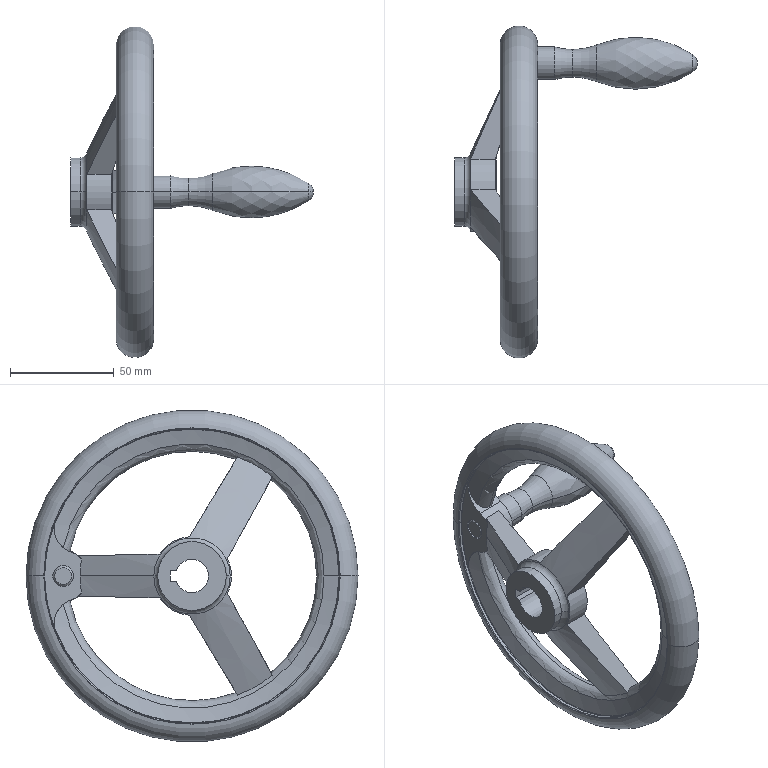Part | STEP file | 1 solid | 72 faces | box 117 x 160 x 160 mm | volume 172381 mm3 | torus 26 | cylinder 19 | plane 14 | cone 9 | other 2 | sphere 2 | commonest cylinder face diameters 33 x4 142 x4 38 x3 10 x2 15.8 x2 24 x2